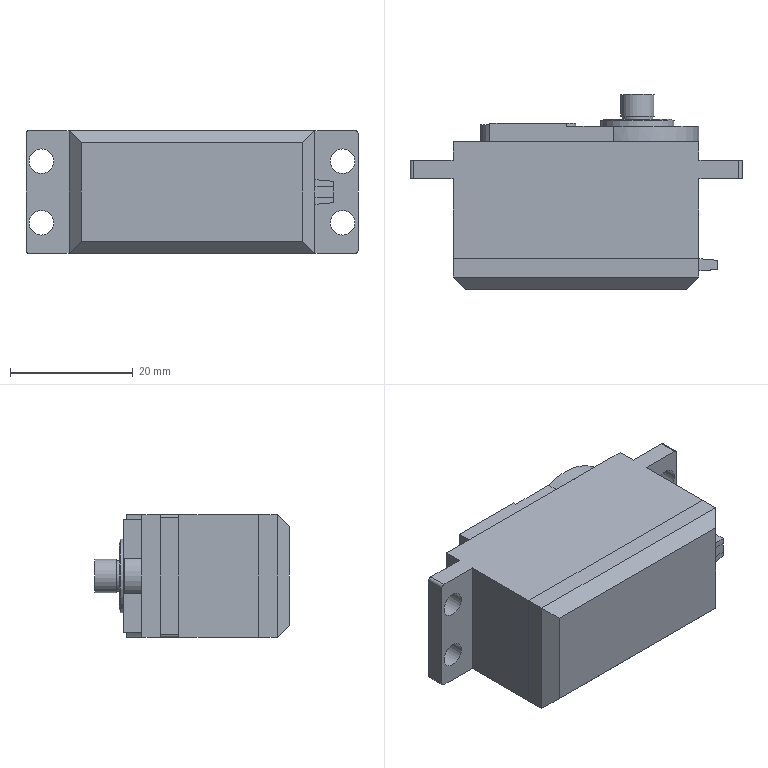Part | STEP file | Huisheng 995 servo-Y | 1 solid | 179 faces | box 54 x 31.7 x 20 mm | volume 21472 mm3 | plane 103 | spline 60 | cylinder 16 | commonest cylinder face diameters 4 x5 1 x4 3 x1 5 x1 5.5 x1 7 x1